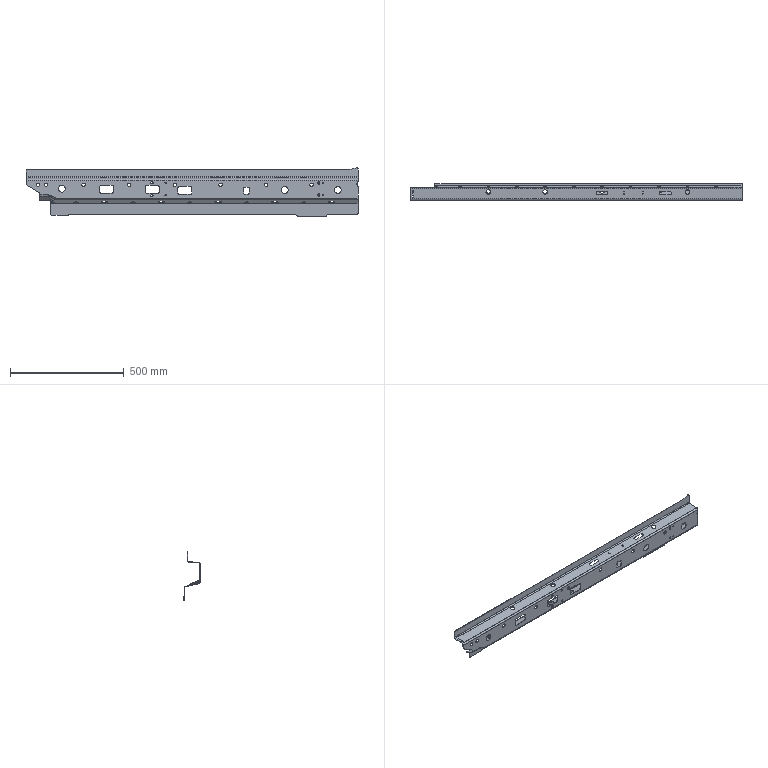Part | STEP file | FNA5401271 | 1 solid | 233 faces | box 1459 x 72.45 x 212.137 mm | volume 599256 mm3 | cylinder 130 | plane 77 | spline 26 | commonest cylinder face diameters 10 x19 20 x18 30 x18 15 x17 2 x16 12 x15